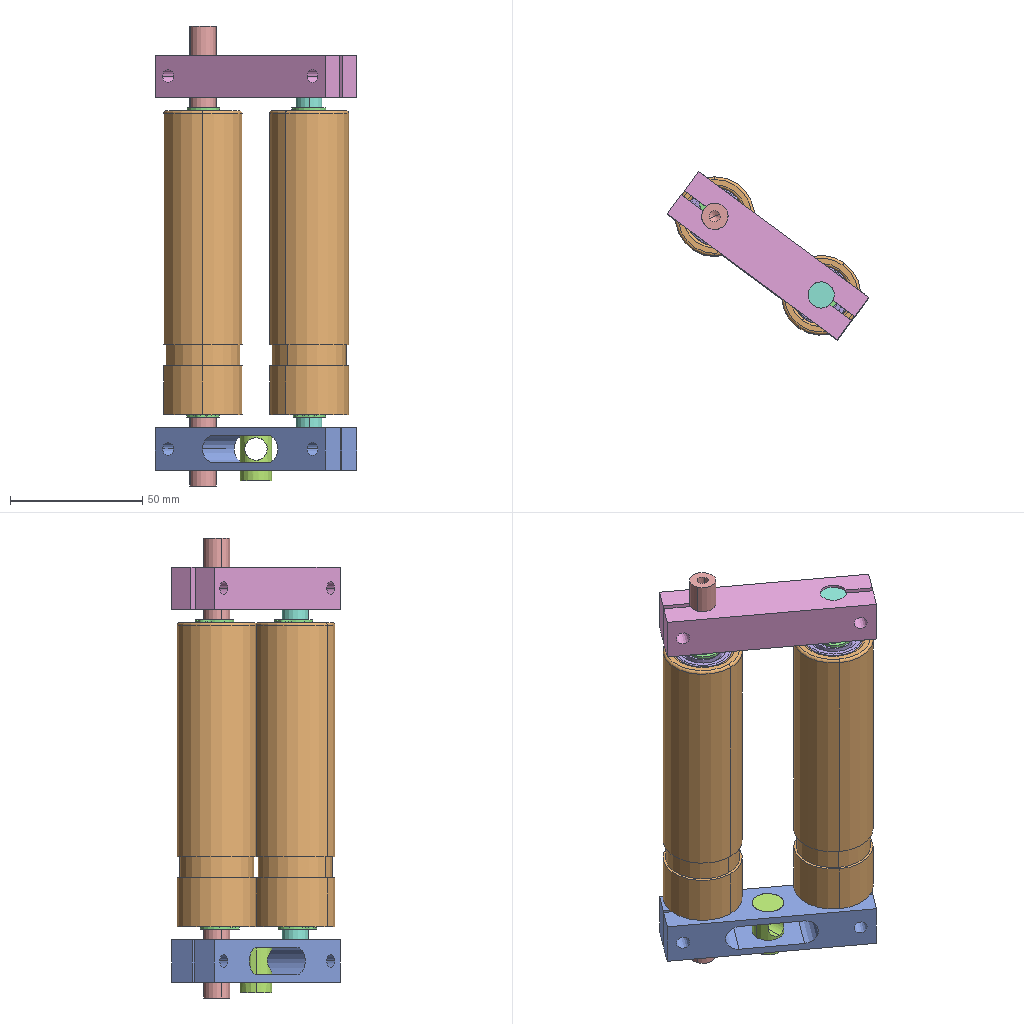Assembly | SolidWorks | 8 different items | 15 placed | box 76 x 64 x 174 mm
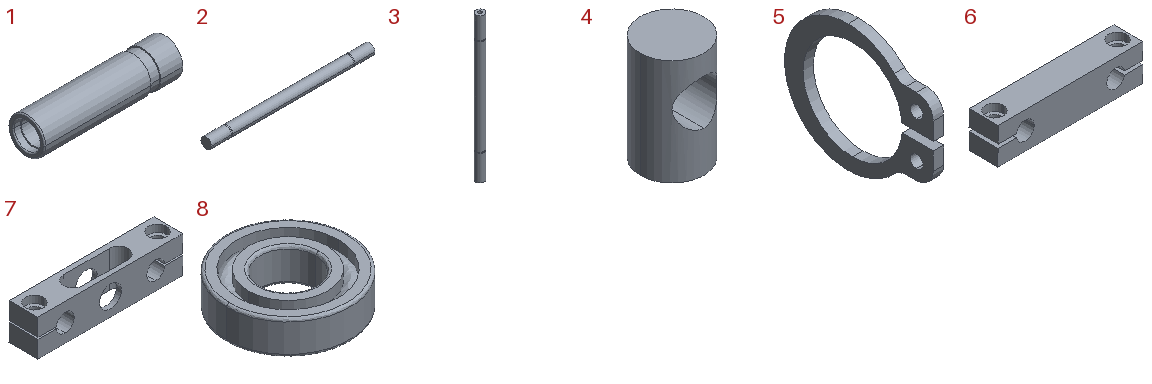Parts list (item | quantity | size | volume | features):
1 | x2 | 115 x 30 x 30 mm | 43595 mm3 | features Fillet 1, Revolution 1
2 | x1 | 155 x 10 x 10 mm | 12160 mm3 | features Revolution 1
3 | x1 | 10 x 10 x 174 mm | 13253 mm3 | features HoleWzd 2, Extrusion 1, RevCut 1
4 | x1 | 12 x 12 x 20 mm | 1627 mm3 | features HoleWzd 2, Extrusion 1
5 | x4 | 1 x 14.4 x 12.3 mm | 59.275 mm3 | features BaseBody 1
6 | x1 | 80 x 16 x 20 mm | 21131 mm3 | features ICE 4, Extrusion 1, HoleWzd 1
7 | x1 | 80 x 16 x 20 mm | 13796 mm3 | features ICE 5, Extrusion 1, HoleWzd 1
8 | x4 | 22 x 22 x 6 mm | 1473 mm3 | features BaseBody 1
Mates (type | each side: item.copy, entity, surface, feature):
Concentric | 3.1 face cylinder Boss-Extrude1 | 7.1 face cylinder Cut-Extrude1
Concentric | 3.1 face cylinder Boss-Extrude1 | 6.1 face cylinder Cut-Extrude1
Coincident | 3.1 face plane Cut-Revolve1 | 2.1 face plane Revolve1
Concentric | 7.1 face cylinder Cut-Extrude2 | 4.1 face cylinder Boss-Extrude1
Coincident | 7.1 face plane Boss-Extrude1 | 4.1 face plane Boss-Extrude1
Coincident | 7.1 face plane Boss-Extrude1 | 6.1 face plane Boss-Extrude1
Concentric | 7.1 face cylinder Cut-Extrude1 | 2.1 face cylinder Revolve1
Concentric | 2.1 face cylinder Revolve1 | 8.1 face cylinder Input1
Coincident | 1.1 face plane Revolve1 | 8.1 face plane Input1
Concentric | 3.1 face cylinder Boss-Extrude1 | 8.2 face cylinder Input1
Coincident | 1.2 face plane Revolve1 | 8.2 face plane Input1
Coincident | 3.1 face plane Cut-Revolve1 | 5.1 face plane Input1
Concentric | 3.1 face cylinder Cut-Revolve1 | 5.1 face cylinder Input1
Concentric | 8.1 face cylinder Input1 | 5.2 face cylinder Input1
Coincident | 8.1 face plane Input1 | 5.2 face plane Input1
Concentric | 5.3 face cylinder Input1 | 8.3 face cylinder Input1
Coincident | 5.3 face plane Input1 | 8.3 face plane Input1
Concentric | 2.1 face cylinder Revolve1 | 8.3 face cylinder Input1
Coincident | 1.1 face plane Revolve1 | 8.3 face plane Input1
Concentric | 5.4 face cylinder Input1 | 8.4 face cylinder Input1
Coincident | 5.4 face plane Input1 | 8.4 face plane Input1
Concentric | 3.1 face cylinder Boss-Extrude1 | 8.4 face cylinder Input1
Coincident | 1.2 face plane Revolve1 | 8.4 face plane Input1